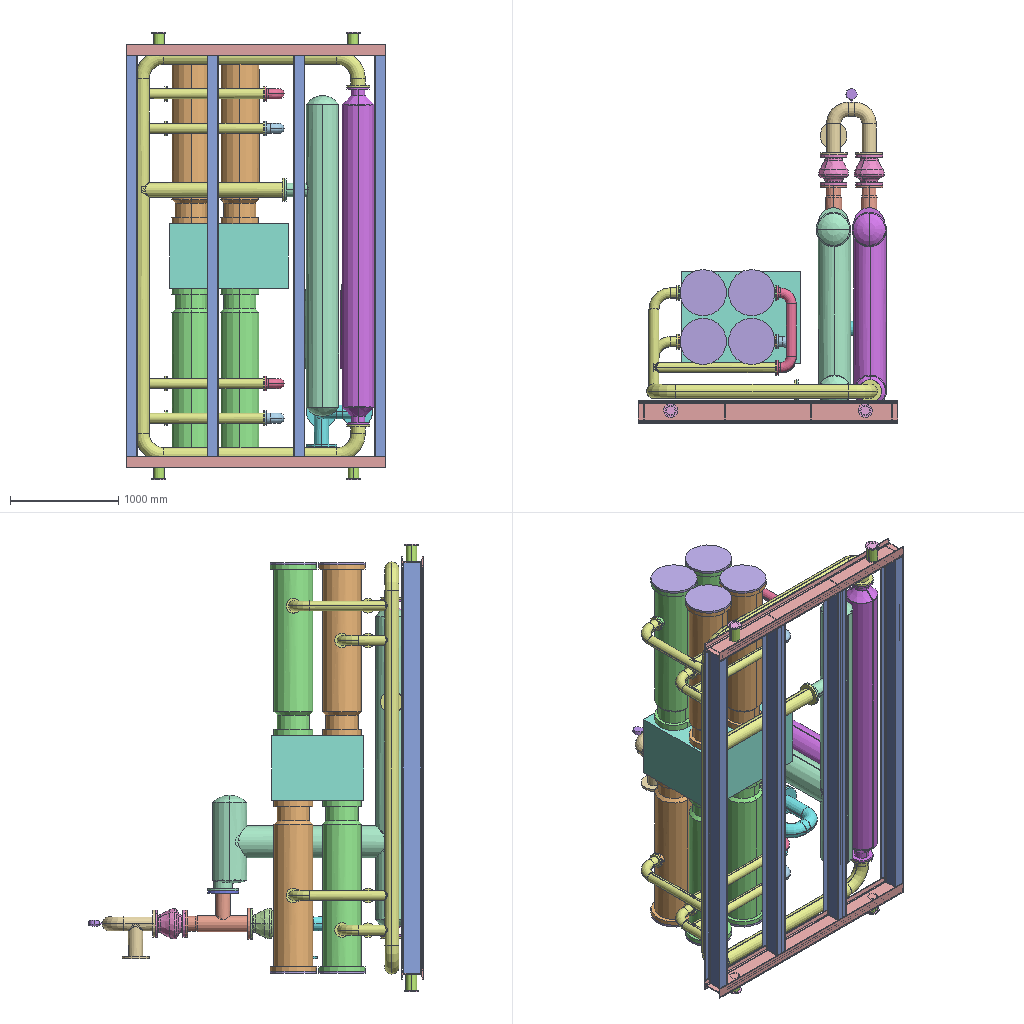Assembly | SolidWorks | 22 different items | 56 placed | box 2400 x 3092 x 4138 mm
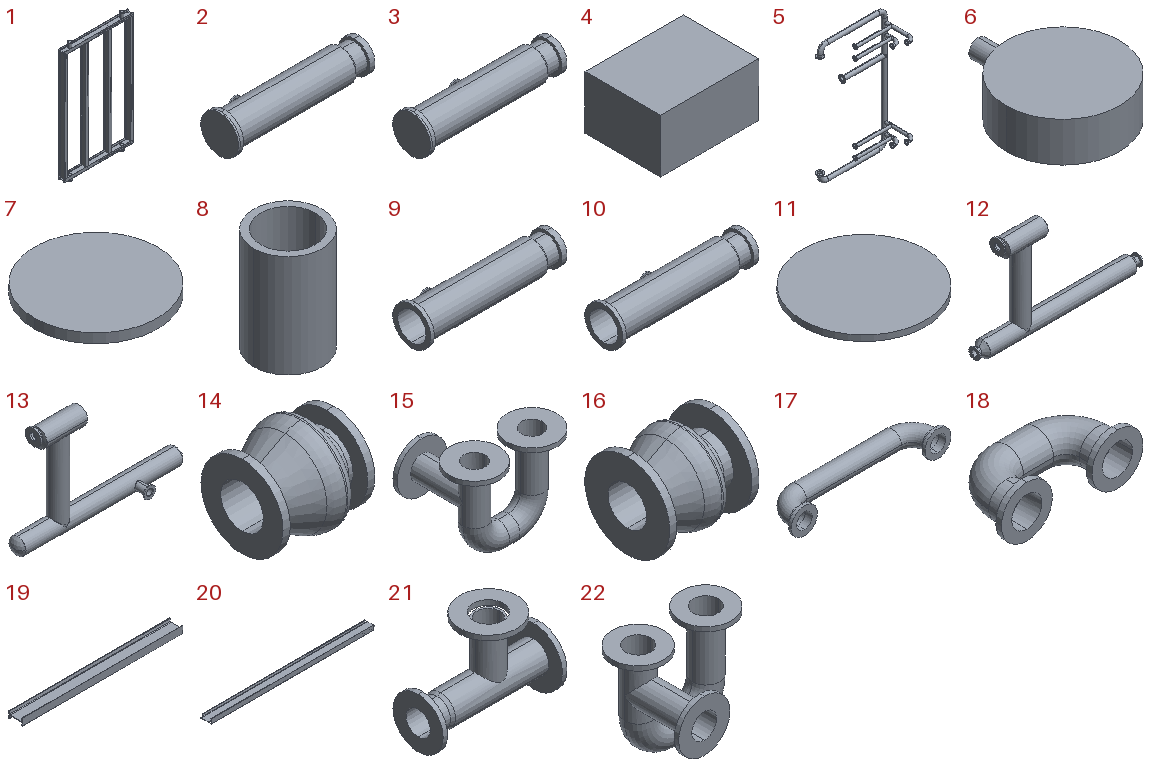Parts list (item | name | quantity | parent item | size | volume | features):
1 | (subassembly) | x1 | - | 2400 x 200 x 4138 mm | 77707667 mm3 | -
2 | (subassembly) | x4 | - | 1600 x 445 x 430 mm | 39813580 mm3 | -
3 | (subassembly) | x4 | - | 1600 x 445 x 430 mm | 39813585 mm3 | -
4 | - | x1 | - | 1100 x 850 x 600 mm | 561000000 mm3 | features Extrusion 1
5 | - | x1 | - | 2172 x 1083 x 3813 mm | 36791331 mm3 | features ICE 9, LPattern 3, Sweep 2
6 | - | x1 | - | 100 x 125 x 35 mm | 279948 mm3 | features Extrusion 1, ICE 1
7 | - | x4 | in 1 | 130 x 130 x 10 mm | 132732 mm3 | features Extrusion 1
8 | - | x4 | in 1 | 100 x 100 x 150 mm | 424115 mm3 | features Extrusion 1
9 | - | x4 | in 2 | 1580 x 445 x 430 mm | 36909179 mm3 | features ICE 4, Revolution 1
10 | - | x4 | in 3 | 1580 x 445 x 430 mm | 36909184 mm3 | features ICE 4, Revolution 1
11 | - | x8 | in 2, 3 | 430 x 430 x 20 mm | 2904402 mm3 | features Extrusion 1
12 | - | x1 | - | 3124 x 319.547 x 1852 mm | 52039073 mm3 | features ICE 3, Revolution 2
13 | - | x1 | - | 2968 x 502 x 1852 mm | 51909646 mm3 | features ICE 5, Revolution 2
14 | - | x2 | - | 280 x 279.772 x 279.772 mm | 7581960 mm3 | features Revolution 1
15 | - | x1 | - | 615 x 466.5 x 490.5 mm | 6883976 mm3 | features ICE 3, Sweep 1
16 | - | x2 | - | 300 x 285 x 285 mm | 8540460 mm3 | features Revolution 1
17 | - | x2 | - | 825 x 181 x 135 mm | 1647054 mm3 | features ICE 1, Sweep 1
18 | - | x2 | - | 375 x 181 x 135 mm | 945407 mm3 | features ICE 1, Sweep 1
19 | - | x2 | in 1 | 2400 x 200 x 102 mm | 9158318 mm3 | features Fillet 2, Extrusion 1
20 | - | x4 | in 1 | 3800 x 200 x 102 mm | 14290911 mm3 | features Fillet 2, ICE 2, Extrusion 1
21 | - | x2 | - | 600 x 285 x 446.5 mm | 7468872 mm3 | features ICE 2, Revolution 1
22 | - | x1 | - | 580 x 447 x 488.5 mm | 5598640 mm3 | features ICE 3, 3DProfileFeature 1, HoleWzd 1, Sweep 1
Mates (type | each side: item.copy, entity, surface, feature):
In the top assembly
DistanceDim | 4.1 face plane Boss-Extrude1 | 19.1 face plane Base
DistanceDim | 19.2 face plane Base | 4.1 face plane Boss-Extrude1
Coincident | 4.1 face plane Boss-Extrude1 | 10.1 face plane Revolve1
Coincident | 4.1 face plane Boss-Extrude1 | 10.2 face plane Revolve1
Coincident | 4.1 face plane Boss-Extrude1 | 9.1 face plane Revolve1
Coincident | 4.1 face plane Boss-Extrude1 | 9.2 face plane Revolve1
Coincident | 4.1 face plane Boss-Extrude1 | 10.3 face plane Revolve1
Coincident | 4.1 face plane Boss-Extrude1 | 10.4 face plane Revolve1
Coincident | 4.1 face plane Boss-Extrude1 | 9.3 face plane Revolve1
DistanceDim | 9.1 select_type:24 | 4.1 face plane Boss-Extrude1 | 2 times
Coincident | 10.1 select_type:24 | 9.1 select_type:24
DistanceDim | 10.1 select_type:24 | 4.1 face plane Boss-Extrude1
Coincident | 9.1 select_type:24 | 9.2 select_type:24
DistanceDim | 9.2 select_type:24 | 9.1 select_type:24
Coincident | 10.2 select_type:24 | 9.2 select_type:24
Coincident | 10.1 select_type:24 | 10.2 select_type:24
DistanceDim | 4.1 face plane Boss-Extrude1 | 19.2 face plane Base
Coincident | 4.1 face plane Boss-Extrude1 | 9.4 face plane Revolve1
DistanceDim | 9.4 select_type:24 | 4.1 face plane Boss-Extrude1
DistanceDim | 9.4 select_type:24 | 9.3 select_type:24
Coincident | 10.4 select_type:24 | 9.4 select_type:24
DistanceDim | 10.4 select_type:24 | 4.1 face plane Boss-Extrude1
Coincident | 10.3 select_type:24 | 10.4 select_type:24
DistanceDim | 10.3 select_type:24 | 4.1 face plane Boss-Extrude1
DistanceDim | 9.3 select_type:24 | 4.1 face plane Boss-Extrude1 | 2 times
Concentric | 9.2 face cylinder Boss-Extrude2 | 17.1 face cylinder Boss-Extrude1
Coincident | 9.2 face plane Boss-Extrude2 | 17.1 face plane Boss-Extrude1
Parallel | 20.1 face plane Base | 17.1 select_type:24
Concentric | 10.4 face cylinder Boss-Extrude2 | 17.2 face cylinder Boss-Extrude1
Parallel | 20.2 face plane Base | 17.2 select_type:24
Concentric | 10.2 face cylinder Boss-Extrude2 | 18.1 face cylinder Boss-Extrude1
Coincident | 10.2 face plane Boss-Extrude2 | 18.1 face plane Boss-Extrude1
Parallel | 20.2 face plane Base | 18.1 select_type:24
Concentric | 9.4 face cylinder Boss-Extrude2 | 18.2 face cylinder Boss-Extrude1
Coincident | 9.4 face plane Boss-Extrude2 | 18.2 face plane Boss-Extrude1
Parallel | 20.2 face plane Base | 18.2 select_type:24
DistanceDim | 5.1 select_type:24 | 20.3 face plane Base
Parallel | 4.1 edge | 5.1 select_type:24
DistanceDim | 5.1 face plane Boss-Extrude2 | 4.1 face plane Boss-Extrude1
Coincident | 5.1 face plane Boss-Extrude2 | 12.1 face plane Revolve1
Concentric | 5.1 face cylinder Boss-Extrude2 | 12.1 face cylinder Revolve1
DistanceDim | 5.1 select_type:24 | 19.2 face plane Base
Parallel | 19.1 edge | 12.1 select_type:24
Coincident | 5.1 face plane Boss-Extrude9 | 13.1 face plane Boss-Extrude5
Concentric | 5.1 face cylinder Boss-Extrude8 | 13.1 face cylinder Boss-Extrude4
Coincident | 10.4 face plane Boss-Extrude2 | 17.2 face plane Boss-Extrude1
Concentric | 12.1 face cylinder Boss-Extrude3 | 21.1 face cylinder Boss-Extrude2
Coincident | 12.1 face plane Boss-Extrude3 | 21.1 face plane Boss-Extrude2
Concentric | 13.1 face cylinder Boss-Extrude3 | 21.2 face cylinder Boss-Extrude2
Coincident | 13.1 face plane Boss-Extrude3 | 21.2 face plane Boss-Extrude2
Parallel | 20.3 face plane Base | 21.1 face plane Revolve1
Parallel | 21.1 face plane Revolve1 | 21.2 face plane Revolve1
Coincident | 21.2 face plane Revolve1 | 16.1 face plane Revolve1
Concentric | 21.2 face cylinder Revolve1 | 16.1 face cylinder Revolve1
Coincident | 21.1 face plane Revolve1 | 16.2 face plane Revolve1
Concentric | 21.1 face cylinder Revolve1 | 16.2 face cylinder Revolve1
Concentric | 21.1 face cylinder Revolve1 | 14.1 face cylinder Revolve1
Coincident | 21.1 face plane Revolve1 | 14.1 face plane Revolve1
Coincident | 21.2 face plane Revolve1 | 14.2 face plane Revolve1
Concentric | 21.2 face cylinder Revolve1 | 14.2 face cylinder Revolve1
Coincident | 16.1 face plane Revolve1 | 15.1 face plane Boss-Extrude1
Concentric | 16.2 face cylinder Revolve1 | 15.1 face cylinder Boss-Extrude1
Parallel | 4.1 face plane Boss-Extrude1 | 15.1 face plane Boss-Extrude3
Coincident | 14.1 face plane Revolve1 | 22.1 face plane Boss-Extrude1
Concentric | 14.2 face cylinder Revolve1 | 22.1 face cylinder Boss-Extrude1
Parallel | 4.1 face plane Boss-Extrude1 | 22.1 face plane Boss-Extrude3
Concentric | 22.1 face cylinder M16 Tapped Hole3 | 6.1 face cylinder Boss-Extrude2
In subassembly 3
Coincident | 10.5 face plane Revolve1 | 11.1 face plane Boss-Extrude1
Concentric | 10.5 face cylinder Revolve1 | 11.1 face cylinder Boss-Extrude1
In subassembly 2
Coincident | 9.5 face plane Revolve1 | 11.1 face plane Boss-Extrude1
Concentric | 9.5 face cylinder Revolve1 | 11.1 face cylinder Boss-Extrude1
In subassembly 1
Coincident | 19.3 face plane Base | 19.4 face plane Base | 2 times
DistanceDim | 19.3 face plane Base | 19.4 face plane Base
Coincident | 19.4 face plane Base | 20.4 face plane Base
Coincident | 19.3 face plane Base | 20.4 face plane Base | 2 times
Coincident | 19.3 face plane Base | 20.5 face plane Base
Coincident | 19.4 face plane Base | 20.5 face plane Base | 2 times
Coincident | 19.3 face plane Base | 8.1 face plane Boss-Extrude1
DistanceDim | 8.1 select_type:24 | 19.3 face plane Base | 2 times
Coincident | 8.1 face plane Boss-Extrude1 | 8.2 face plane Boss-Extrude1
Coincident | 8.1 select_type:24 | 8.2 select_type:24
DistanceDim | 8.2 select_type:24 | 19.3 face plane Base
Coincident | 19.4 face plane Base | 8.3 face plane Boss-Extrude1
Coincident | 8.3 face plane Boss-Extrude1 | 8.4 face plane Boss-Extrude1
Coincident | 8.3 select_type:24 | 8.4 select_type:24
DistanceDim | 8.3 select_type:24 | 19.4 face plane Base | 2 times
DistanceDim | 8.4 select_type:24 | 19.4 face plane Base
Concentric | 8.4 face cylinder Boss-Extrude1 | 7.1 face cylinder Boss-Extrude1
Coincident | 8.4 face plane Boss-Extrude1 | 7.1 face plane Boss-Extrude1
Concentric | 8.3 face cylinder Boss-Extrude1 | 7.2 face cylinder Boss-Extrude1
Coincident | 8.3 face plane Boss-Extrude1 | 7.2 face plane Boss-Extrude1
Concentric | 8.2 face cylinder Boss-Extrude1 | 7.3 face cylinder Boss-Extrude1
Coincident | 8.2 face plane Boss-Extrude1 | 7.3 face plane Boss-Extrude1
Concentric | 8.1 face cylinder Boss-Extrude1 | 7.4 face cylinder Boss-Extrude1
Coincident | 8.1 face plane Boss-Extrude1 | 7.4 face plane Boss-Extrude1
Coincident | 19.4 face plane Base | 20.6 face plane Base | 2 times
DistanceDim | 20.6 face plane Base | 20.5 face plane Base
Coincident | 19.4 face plane Base | 20.7 face plane Base | 2 times
DistanceDim | 20.7 face plane Base | 19.4 face plane Base